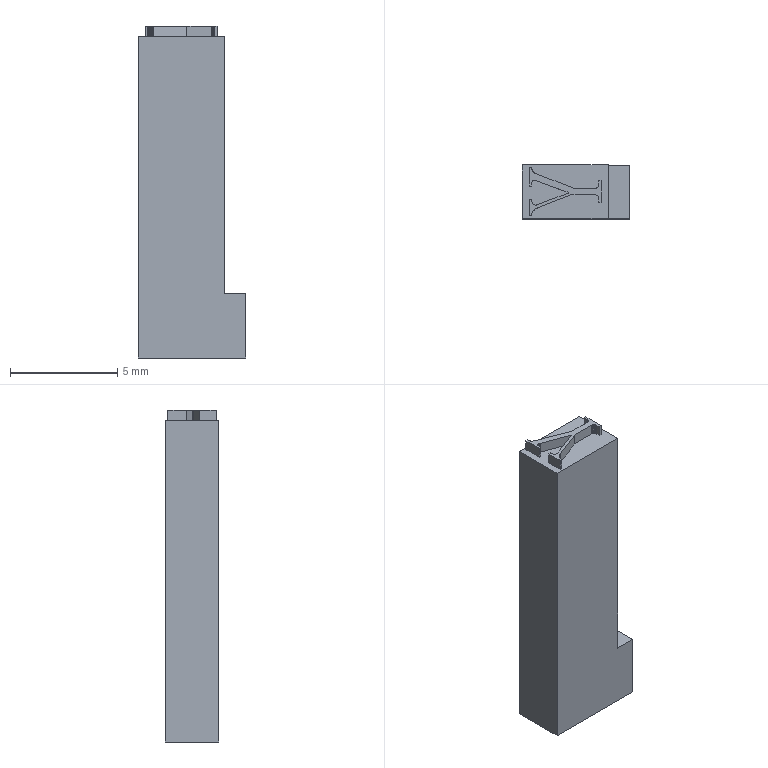Part | NX | features DIE-18 2 | 1 solid | 89 faces | box 5 x 2.5 x 15.5 mm | volume 158.298 mm3 | plane 89